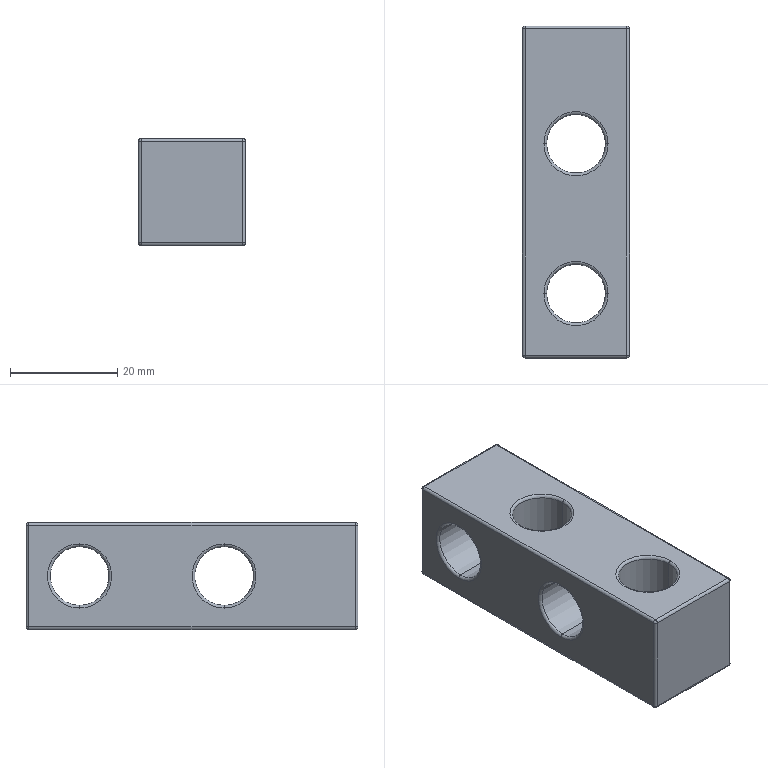Part | SolidWorks | features Extrusion 1, Fillet 1, ICE 1 | 1 solid | 50 faces | box 20 x 62 x 20 mm | volume 17160 mm3 | cylinder 20 | torus 16 | sphere 8 | plane 6 | commonest cylinder face diameters 1 x12 11 x8
STEP:
#1=CARTESIAN_POINT('',(-6.,-19.,10.));
#2=VERTEX_POINT('',#1);
#3=CARTESIAN_POINT('',(6.,-19.,10.));
#4=VERTEX_POINT('',#3);
#5=CARTESIAN_POINT('',(0.,-19.,10.));
#6=DIRECTION('',(0.,0.,-1.));
#7=DIRECTION('',(1.,0.,0.));
#8=AXIS2_PLACEMENT_3D('',#5,#6,#7);
#9=CIRCLE('',#8,6.);
#10=EDGE_CURVE('',#2,#4,#9,.T.);
#11=ORIENTED_EDGE('',*,*,#10,.F.);
#12=CARTESIAN_POINT('',(-5.5,-19.,9.5));
#13=VERTEX_POINT('',#12);
#14=CARTESIAN_POINT('',(-6.,-19.,9.5));
#15=DIRECTION('',(0.,1.,0.));
#16=DIRECTION('',(-1.,0.,0.));
#17=AXIS2_PLACEMENT_3D('',#14,#15,#16);
#18=CIRCLE('',#17,0.5);
#19=EDGE_CURVE('',#2,#13,#18,.T.);
#20=ORIENTED_EDGE('',*,*,#19,.T.);
#21=CARTESIAN_POINT('',(5.5,-19.,9.5));
#22=VERTEX_POINT('',#21);
#23=CARTESIAN_POINT('',(0.,-19.,9.5));
#24=DIRECTION('',(0.,0.,1.));
#25=DIRECTION('',(1.,0.,0.));
#26=AXIS2_PLACEMENT_3D('',#23,#24,#25);
#27=CIRCLE('',#26,5.5);
#28=EDGE_CURVE('',#22,#13,#27,.T.);
#29=ORIENTED_EDGE('',*,*,#28,.F.);
#30=CARTESIAN_POINT('',(6.,-19.,9.5));
#31=DIRECTION('',(0.,-1.,0.));
#32=DIRECTION('',(0.,0.,-1.));
#33=AXIS2_PLACEMENT_3D('',#30,#31,#32);
#34=CIRCLE('',#33,0.5);
#35=EDGE_CURVE('',#4,#22,#34,.T.);
#36=ORIENTED_EDGE('',*,*,#35,.F.);
#37=EDGE_LOOP('',(#11,#20,#29,#36));
#38=FACE_OUTER_BOUND('',#37,.T.);
#39=CARTESIAN_POINT('',(0.,-19.,9.5));
#40=DIRECTION('',(0.,0.,1.));
#41=DIRECTION('',(1.,0.,0.));
#42=AXIS2_PLACEMENT_3D('',#39,#40,#41);
#43=TOROIDAL_SURFACE('',#42,6.,0.5);
#44=ADVANCED_FACE('',(#38),#43,.T.);
#45=CARTESIAN_POINT('',(-6.,9.,10.));
#46=VERTEX_POINT('',#45);
#47=CARTESIAN_POINT('',(6.,9.,10.));
#48=VERTEX_POINT('',#47);
#49=CARTESIAN_POINT('',(0.,9.,10.));
#50=DIRECTION('',(0.,0.,-1.));
#51=DIRECTION('',(1.,0.,0.));
#52=AXIS2_PLACEMENT_3D('',#49,#50,#51);
#53=CIRCLE('',#52,6.);
#54=EDGE_CURVE('',#46,#48,#53,.T.);
#55=ORIENTED_EDGE('',*,*,#54,.F.);
#56=CARTESIAN_POINT('',(-5.5,9.,9.5));
#57=VERTEX_POINT('',#56);
#58=CARTESIAN_POINT('',(-6.,9.,9.5));
#59=DIRECTION('',(0.,1.,0.));
#60=DIRECTION('',(-1.,0.,0.));
#61=AXIS2_PLACEMENT_3D('',#58,#59,#60);
#62=CIRCLE('',#61,0.5);
#63=EDGE_CURVE('',#46,#57,#62,.T.);
#64=ORIENTED_EDGE('',*,*,#63,.T.);
#65=CARTESIAN_POINT('',(5.5,9.,9.5));
#66=VERTEX_POINT('',#65);
#67=CARTESIAN_POINT('',(0.,9.,9.5));
#68=DIRECTION('',(0.,0.,1.));
#69=DIRECTION('',(1.,0.,0.));
#70=AXIS2_PLACEMENT_3D('',#67,#68,#69);
#71=CIRCLE('',#70,5.5);
#72=EDGE_CURVE('',#66,#57,#71,.T.);
#73=ORIENTED_EDGE('',*,*,#72,.F.);
#74=CARTESIAN_POINT('',(6.,9.,9.5));
#75=DIRECTION('',(0.,-1.,0.));
#76=DIRECTION('',(0.,0.,-1.));
#77=AXIS2_PLACEMENT_3D('',#74,#75,#76);
#78=CIRCLE('',#77,0.5);
#79=EDGE_CURVE('',#48,#66,#78,.T.);
#80=ORIENTED_EDGE('',*,*,#79,.F.);
#81=EDGE_LOOP('',(#55,#64,#73,#80));
#82=FACE_OUTER_BOUND('',#81,.T.);
#83=CARTESIAN_POINT('',(0.,9.,9.5));
#84=DIRECTION('',(0.,0.,1.));
#85=DIRECTION('',(1.,0.,0.));
#86=AXIS2_PLACEMENT_3D('',#83,#84,#85);
#87=TOROIDAL_SURFACE('',#86,6.,0.5);
#88=ADVANCED_FACE('',(#82),#87,.T.);
#89=CARTESIAN_POINT('',(9.5,-6.,-5.5));
#90=VERTEX_POINT('',#89);
#91=CARTESIAN_POINT('',(9.5,-6.,5.5));
#92=VERTEX_POINT('',#91);
#93=CARTESIAN_POINT('',(9.5,-6.,0.));
#94=DIRECTION('',(1.,0.,0.));
#95=DIRECTION('',(0.,0.,1.));
#96=AXIS2_PLACEMENT_3D('',#93,#94,#95);
#97=CIRCLE('',#96,5.5);
#98=EDGE_CURVE('',#90,#92,#97,.T.);
#99=ORIENTED_EDGE('',*,*,#98,.F.);
#100=CARTESIAN_POINT('',(10.,-6.,-6.));
#101=VERTEX_POINT('',#100);
#102=CARTESIAN_POINT('',(9.5,-6.,-6.));
#103=DIRECTION('',(0.,1.,0.));
#104=DIRECTION('',(0.,0.,1.));
#105=AXIS2_PLACEMENT_3D('',#102,#103,#104);
#106=CIRCLE('',#105,0.5);
#107=EDGE_CURVE('',#90,#101,#106,.T.);
#108=ORIENTED_EDGE('',*,*,#107,.T.);
#109=CARTESIAN_POINT('',(10.,-6.,6.));
#110=VERTEX_POINT('',#109);
#111=CARTESIAN_POINT('',(10.,-6.,0.));
#112=DIRECTION('',(-1.,0.,0.));
#113=DIRECTION('',(0.,0.,1.));
#114=AXIS2_PLACEMENT_3D('',#111,#112,#113);
#115=CIRCLE('',#114,6.);
#116=EDGE_CURVE('',#110,#101,#115,.T.);
#117=ORIENTED_EDGE('',*,*,#116,.F.);
#118=CARTESIAN_POINT('',(9.5,-6.,6.));
#119=DIRECTION('',(0.,-1.,0.));
#120=DIRECTION('',(0.,0.,-1.));
#121=AXIS2_PLACEMENT_3D('',#118,#119,#120);
#122=CIRCLE('',#121,0.5);
#123=EDGE_CURVE('',#92,#110,#122,.T.);
#124=ORIENTED_EDGE('',*,*,#123,.F.);
#125=EDGE_LOOP('',(#99,#108,#117,#124));
#126=FACE_OUTER_BOUND('',#125,.T.);
#127=CARTESIAN_POINT('',(9.5,-6.,0.));
#128=DIRECTION('',(-1.,0.,0.));
#129=DIRECTION('',(0.,0.,1.));
#130=AXIS2_PLACEMENT_3D('',#127,#128,#129);
#131=TOROIDAL_SURFACE('',#130,6.,0.5);
#132=ADVANCED_FACE('',(#126),#131,.T.);
#133=CARTESIAN_POINT('',(9.5,21.,-5.5));
#134=VERTEX_POINT('',#133);
#135=CARTESIAN_POINT('',(9.5,21.,5.5));
#136=VERTEX_POINT('',#135);
#137=CARTESIAN_POINT('',(9.5,21.,0.));
#138=DIRECTION('',(1.,0.,0.));
#139=DIRECTION('',(0.,0.,1.));
#140=AXIS2_PLACEMENT_3D('',#137,#138,#139);
#141=CIRCLE('',#140,5.5);
#142=EDGE_CURVE('',#134,#136,#141,.T.);
#143=ORIENTED_EDGE('',*,*,#142,.F.);
#144=CARTESIAN_POINT('',(10.,21.,-6.));
#145=VERTEX_POINT('',#144);
#146=CARTESIAN_POINT('',(9.5,21.,-6.));
#147=DIRECTION('',(0.,1.,0.));
#148=DIRECTION('',(0.,0.,1.));
#149=AXIS2_PLACEMENT_3D('',#146,#147,#148);
#150=CIRCLE('',#149,0.5);
#151=EDGE_CURVE('',#134,#145,#150,.T.);
#152=ORIENTED_EDGE('',*,*,#151,.T.);
#153=CARTESIAN_POINT('',(10.,21.,6.));
#154=VERTEX_POINT('',#153);
#155=CARTESIAN_POINT('',(10.,21.,0.));
#156=DIRECTION('',(-1.,0.,0.));
#157=DIRECTION('',(0.,0.,1.));
#158=AXIS2_PLACEMENT_3D('',#155,#156,#157);
#159=CIRCLE('',#158,6.);
#160=EDGE_CURVE('',#154,#145,#159,.T.);
#161=ORIENTED_EDGE('',*,*,#160,.F.);
#162=CARTESIAN_POINT('',(9.5,21.,6.));
#163=DIRECTION('',(0.,-1.,0.));
#164=DIRECTION('',(0.,0.,-1.));
#165=AXIS2_PLACEMENT_3D('',#162,#163,#164);
#166=CIRCLE('',#165,0.5);
#167=EDGE_CURVE('',#136,#154,#166,.T.);
#168=ORIENTED_EDGE('',*,*,#167,.F.);
#169=EDGE_LOOP('',(#143,#152,#161,#168));
#170=FACE_OUTER_BOUND('',#169,.T.);
#171=CARTESIAN_POINT('',(9.5,21.,0.));
#172=DIRECTION('',(-1.,0.,0.));
#173=DIRECTION('',(0.,0.,1.));
#174=AXIS2_PLACEMENT_3D('',#171,#172,#173);
#175=TOROIDAL_SURFACE('',#174,6.,0.5);
#176=ADVANCED_FACE('',(#170),#175,.T.);
#177=CARTESIAN_POINT('',(-5.5,-19.,-9.5));
#178=VERTEX_POINT('',#177);
#179=CARTESIAN_POINT('',(5.5,-19.,-9.5));
#180=VERTEX_POINT('',#179);
#181=CARTESIAN_POINT('',(0.,-19.,-9.5));
#182=DIRECTION('',(0.,0.,-1.));
#183=DIRECTION('',(1.,0.,0.));
#184=AXIS2_PLACEMENT_3D('',#181,#182,#183);
#185=CIRCLE('',#184,5.5);
#186=EDGE_CURVE('',#178,#180,#185,.T.);
#187=ORIENTED_EDGE('',*,*,#186,.F.);
#188=CARTESIAN_POINT('',(-6.,-19.,-10.));
#189=VERTEX_POINT('',#188);
#190=CARTESIAN_POINT('',(-6.,-19.,-9.5));
#191=DIRECTION('',(0.,1.,0.));
#192=DIRECTION('',(-1.,0.,0.));
#193=AXIS2_PLACEMENT_3D('',#190,#191,#192);
#194=CIRCLE('',#193,0.5);
#195=EDGE_CURVE('',#178,#189,#194,.T.);
#196=ORIENTED_EDGE('',*,*,#195,.T.);
#197=CARTESIAN_POINT('',(6.,-19.,-10.));
#198=VERTEX_POINT('',#197);
#199=CARTESIAN_POINT('',(0.,-19.,-10.));
#200=DIRECTION('',(0.,0.,1.));
#201=DIRECTION('',(1.,0.,0.));
#202=AXIS2_PLACEMENT_3D('',#199,#200,#201);
#203=CIRCLE('',#202,6.);
#204=EDGE_CURVE('',#198,#189,#203,.T.);
#205=ORIENTED_EDGE('',*,*,#204,.F.);
#206=CARTESIAN_POINT('',(6.,-19.,-9.5));
#207=DIRECTION('',(0.,-1.,0.));
#208=DIRECTION('',(0.,0.,-1.));
#209=AXIS2_PLACEMENT_3D('',#206,#207,#208);
#210=CIRCLE('',#209,0.5);
#211=EDGE_CURVE('',#180,#198,#210,.T.);
#212=ORIENTED_EDGE('',*,*,#211,.F.);
#213=EDGE_LOOP('',(#187,#196,#205,#212));
#214=FACE_OUTER_BOUND('',#213,.T.);
#215=CARTESIAN_POINT('',(0.,-19.,-9.5));
#216=DIRECTION('',(0.,0.,1.));
#217=DIRECTION('',(1.,0.,0.));
#218=AXIS2_PLACEMENT_3D('',#215,#216,#217);
#219=TOROIDAL_SURFACE('',#218,6.,0.5);
#220=ADVANCED_FACE('',(#214),#219,.T.);
#221=CARTESIAN_POINT('',(-5.5,9.,-9.5));
#222=VERTEX_POINT('',#221);
#223=CARTESIAN_POINT('',(5.5,9.,-9.5));
#224=VERTEX_POINT('',#223);
#225=CARTESIAN_POINT('',(0.,9.,-9.5));
#226=DIRECTION('',(0.,0.,-1.));
#227=DIRECTION('',(1.,0.,0.));
#228=AXIS2_PLACEMENT_3D('',#225,#226,#227);
#229=CIRCLE('',#228,5.5);
#230=EDGE_CURVE('',#222,#224,#229,.T.);
#231=ORIENTED_EDGE('',*,*,#230,.F.);
#232=CARTESIAN_POINT('',(-6.,9.,-10.));
#233=VERTEX_POINT('',#232);
#234=CARTESIAN_POINT('',(-6.,9.,-9.5));
#235=DIRECTION('',(0.,1.,0.));
#236=DIRECTION('',(-1.,0.,0.));
#237=AXIS2_PLACEMENT_3D('',#234,#235,#236);
#238=CIRCLE('',#237,0.5);
#239=EDGE_CURVE('',#222,#233,#238,.T.);
#240=ORIENTED_EDGE('',*,*,#239,.T.);
#241=CARTESIAN_POINT('',(6.,9.,-10.));
#242=VERTEX_POINT('',#241);
#243=CARTESIAN_POINT('',(0.,9.,-10.));
#244=DIRECTION('',(0.,0.,1.));
#245=DIRECTION('',(1.,0.,0.));
#246=AXIS2_PLACEMENT_3D('',#243,#244,#245);
#247=CIRCLE('',#246,6.);
#248=EDGE_CURVE('',#242,#233,#247,.T.);
#249=ORIENTED_EDGE('',*,*,#248,.F.);
#250=CARTESIAN_POINT('',(6.,9.,-9.5));
#251=DIRECTION('',(0.,-1.,0.));
#252=DIRECTION('',(0.,0.,-1.));
#253=AXIS2_PLACEMENT_3D('',#250,#251,#252);
#254=CIRCLE('',#253,0.5);
#255=EDGE_CURVE('',#224,#242,#254,.T.);
#256=ORIENTED_EDGE('',*,*,#255,.F.);
#257=EDGE_LOOP('',(#231,#240,#249,#256));
#258=FACE_OUTER_BOUND('',#257,.T.);
#259=CARTESIAN_POINT('',(0.,9.,-9.5));
#260=DIRECTION('',(0.,0.,1.));
#261=DIRECTION('',(1.,0.,0.));
#262=AXIS2_PLACEMENT_3D('',#259,#260,#261);
#263=TOROIDAL_SURFACE('',#262,6.,0.5);
#264=ADVANCED_FACE('',(#258),#263,.T.);
#265=CARTESIAN_POINT('',(-9.5,-6.,5.5));
#266=VERTEX_POINT('',#265);
#267=CARTESIAN_POINT('',(-9.5,-6.,-5.5));
#268=VERTEX_POINT('',#267);
#269=CARTESIAN_POINT('',(-9.5,-6.,0.));
#270=DIRECTION('',(-1.,0.,0.));
#271=DIRECTION('',(0.,0.,-1.));
#272=AXIS2_PLACEMENT_3D('',#269,#270,#271);
#273=CIRCLE('',#272,5.5);
#274=EDGE_CURVE('',#266,#268,#273,.T.);
#275=ORIENTED_EDGE('',*,*,#274,.F.);
#276=CARTESIAN_POINT('',(-10.,-6.,6.));
#277=VERTEX_POINT('',#276);
#278=CARTESIAN_POINT('',(-9.5,-6.,6.));
#279=DIRECTION('',(0.,1.,0.));
#280=DIRECTION('',(0.,0.,1.));
#281=AXIS2_PLACEMENT_3D('',#278,#279,#280);
#282=CIRCLE('',#281,0.5);
#283=EDGE_CURVE('',#266,#277,#282,.T.);
#284=ORIENTED_EDGE('',*,*,#283,.T.);
#285=CARTESIAN_POINT('',(-10.,-6.,-6.));
#286=VERTEX_POINT('',#285);
#287=CARTESIAN_POINT('',(-10.,-6.,0.));
#288=DIRECTION('',(1.,0.,0.));
#289=DIRECTION('',(0.,0.,-1.));
#290=AXIS2_PLACEMENT_3D('',#287,#288,#289);
#291=CIRCLE('',#290,6.);
#292=EDGE_CURVE('',#286,#277,#291,.T.);
#293=ORIENTED_EDGE('',*,*,#292,.F.);
#294=CARTESIAN_POINT('',(-9.5,-6.,-6.));
#295=DIRECTION('',(0.,-1.,0.));
#296=DIRECTION('',(0.,0.,-1.));
#297=AXIS2_PLACEMENT_3D('',#294,#295,#296);
#298=CIRCLE('',#297,0.5);
#299=EDGE_CURVE('',#268,#286,#298,.T.);
#300=ORIENTED_EDGE('',*,*,#299,.F.);
#301=EDGE_LOOP('',(#275,#284,#293,#300));
#302=FACE_OUTER_BOUND('',#301,.T.);
#303=CARTESIAN_POINT('',(-9.5,-6.,0.));
#304=DIRECTION('',(1.,0.,0.));
#305=DIRECTION('',(0.,0.,-1.));
#306=AXIS2_PLACEMENT_3D('',#303,#304,#305);
#307=TOROIDAL_SURFACE('',#306,6.,0.5);
#308=ADVANCED_FACE('',(#302),#307,.T.);
#309=CARTESIAN_POINT('',(-9.5,21.,5.5));
#310=VERTEX_POINT('',#309);
#311=CARTESIAN_POINT('',(-9.5,21.,-5.5));
#312=VERTEX_POINT('',#311);
#313=CARTESIAN_POINT('',(-9.5,21.,0.));
#314=DIRECTION('',(-1.,0.,0.));
#315=DIRECTION('',(0.,0.,-1.));
#316=AXIS2_PLACEMENT_3D('',#313,#314,#315);
#317=CIRCLE('',#316,5.5);
#318=EDGE_CURVE('',#310,#312,#317,.T.);
#319=ORIENTED_EDGE('',*,*,#318,.F.);
#320=CARTESIAN_POINT('',(-10.,21.,6.));
#321=VERTEX_POINT('',#320);
#322=CARTESIAN_POINT('',(-9.5,21.,6.));
#323=DIRECTION('',(0.,1.,0.));
#324=DIRECTION('',(0.,0.,1.));
#325=AXIS2_PLACEMENT_3D('',#322,#323,#324);
#326=CIRCLE('',#325,0.5);
#327=EDGE_CURVE('',#310,#321,#326,.T.);
#328=ORIENTED_EDGE('',*,*,#327,.T.);
#329=CARTESIAN_POINT('',(-10.,21.,-6.));
#330=VERTEX_POINT('',#329);
#331=CARTESIAN_POINT('',(-10.,21.,0.));
#332=DIRECTION('',(1.,0.,0.));
#333=DIRECTION('',(0.,0.,-1.));
#334=AXIS2_PLACEMENT_3D('',#331,#332,#333);
#335=CIRCLE('',#334,6.);
#336=EDGE_CURVE('',#330,#321,#335,.T.);
#337=ORIENTED_EDGE('',*,*,#336,.F.);
#338=CARTESIAN_POINT('',(-9.5,21.,-6.));
#339=DIRECTION('',(0.,-1.,0.));
#340=DIRECTION('',(0.,0.,-1.));
#341=AXIS2_PLACEMENT_3D('',#338,#339,#340);
#342=CIRCLE('',#341,0.5);
#343=EDGE_CURVE('',#312,#330,#342,.T.);
#344=ORIENTED_EDGE('',*,*,#343,.F.);
#345=EDGE_LOOP('',(#319,#328,#337,#344));
#346=FACE_OUTER_BOUND('',#345,.T.);
#347=CARTESIAN_POINT('',(-9.5,21.,0.));
#348=DIRECTION('',(1.,0.,0.));
#349=DIRECTION('',(0.,0.,-1.));
#350=AXIS2_PLACEMENT_3D('',#347,#348,#349);
#351=TOROIDAL_SURFACE('',#350,6.,0.5);
#352=ADVANCED_FACE('',(#346),#351,.T.);
#353=CARTESIAN_POINT('',(-9.5,-6.,0.));
#354=DIRECTION('',(-1.,0.,0.));
#355=DIRECTION('',(0.,0.,-1.));
#356=AXIS2_PLACEMENT_3D('',#353,#354,#355);
#357=CIRCLE('',#356,5.5);
#358=EDGE_CURVE('',#268,#266,#357,.T.);
#359=ORIENTED_EDGE('',*,*,#358,.T.);
#360=CARTESIAN_POINT('',(-10.,-6.,5.5));
#361=DIRECTION('',(1.,0.,0.));
#362=VECTOR('',#361,1000.);
#363=LINE('',#360,#362);
#364=EDGE_CURVE('',#266,#92,#363,.T.);
#365=ORIENTED_EDGE('',*,*,#364,.T.);
#366=CARTESIAN_POINT('',(9.5,-6.,0.));
#367=DIRECTION('',(1.,0.,0.));
#368=DIRECTION('',(0.,0.,1.));
#369=AXIS2_PLACEMENT_3D('',#366,#367,#368);
#370=CIRCLE('',#369,5.5);
#371=EDGE_CURVE('',#92,#90,#370,.T.);
#372=ORIENTED_EDGE('',*,*,#371,.T.);
#373=CARTESIAN_POINT('',(-10.,-6.,-5.5));
#374=DIRECTION('',(1.,0.,0.));
#375=VECTOR('',#374,1000.);
#376=LINE('',#373,#375);
#377=EDGE_CURVE('',#268,#90,#376,.T.);
#378=ORIENTED_EDGE('',*,*,#377,.F.);
#379=EDGE_LOOP('',(#359,#365,#372,#378));
#380=FACE_OUTER_BOUND('',#379,.T.);
#381=CARTESIAN_POINT('',(-10.,-6.,0.));
#382=DIRECTION('',(1.,0.,0.));
#383=DIRECTION('',(0.,0.,-1.));
#384=AXIS2_PLACEMENT_3D('',#381,#382,#383);
#385=CYLINDRICAL_SURFACE('',#384,5.5);
#386=ADVANCED_FACE('',(#380),#385,.F.);
#387=CARTESIAN_POINT('',(-9.5,21.,0.));
#388=DIRECTION('',(-1.,0.,0.));
#389=DIRECTION('',(0.,0.,-1.));
#390=AXIS2_PLACEMENT_3D('',#387,#388,#389);
#391=CIRCLE('',#390,5.5);
#392=EDGE_CURVE('',#312,#310,#391,.T.);
#393=ORIENTED_EDGE('',*,*,#392,.T.);
#394=CARTESIAN_POINT('',(-10.,21.,5.5));
#395=DIRECTION('',(1.,0.,0.));
#396=VECTOR('',#395,1000.);
#397=LINE('',#394,#396);
#398=EDGE_CURVE('',#310,#136,#397,.T.);
#399=ORIENTED_EDGE('',*,*,#398,.T.);
#400=CARTESIAN_POINT('',(9.5,21.,0.));
#401=DIRECTION('',(1.,0.,0.));
#402=DIRECTION('',(0.,0.,1.));
#403=AXIS2_PLACEMENT_3D('',#400,#401,#402);
#404=CIRCLE('',#403,5.5);
#405=EDGE_CURVE('',#136,#134,#404,.T.);
#406=ORIENTED_EDGE('',*,*,#405,.T.);
#407=CARTESIAN_POINT('',(-10.,21.,-5.5));
#408=DIRECTION('',(1.,0.,0.));
#409=VECTOR('',#408,1000.);
#410=LINE('',#407,#409);
#411=EDGE_CURVE('',#312,#134,#410,.T.);
#412=ORIENTED_EDGE('',*,*,#411,.F.);
#413=EDGE_LOOP('',(#393,#399,#406,#412));
#414=FACE_OUTER_BOUND('',#413,.T.);
#415=CARTESIAN_POINT('',(-10.,21.,0.));
#416=DIRECTION('',(1.,0.,0.));
#417=DIRECTION('',(0.,0.,-1.));
#418=AXIS2_PLACEMENT_3D('',#415,#416,#417);
#419=CYLINDRICAL_SURFACE('',#418,5.5);
#420=ADVANCED_FACE('',(#414),#419,.F.);
#421=CARTESIAN_POINT('',(0.,9.,9.5));
#422=DIRECTION('',(0.,0.,1.));
#423=DIRECTION('',(1.,0.,0.));
#424=AXIS2_PLACEMENT_3D('',#421,#422,#423);
#425=CIRCLE('',#424,5.5);
#426=EDGE_CURVE('',#57,#66,#425,.T.);
#427=ORIENTED_EDGE('',*,*,#426,.T.);
#428=CARTESIAN_POINT('',(5.5,9.,10.));
#429=DIRECTION('',(0.,0.,-1.));
#430=VECTOR('',#429,1000.);
#431=LINE('',#428,#430);
#432=EDGE_CURVE('',#66,#224,#431,.T.);
#433=ORIENTED_EDGE('',*,*,#432,.T.);
#434=CARTESIAN_POINT('',(0.,9.,-9.5));
#435=DIRECTION('',(0.,0.,-1.));
#436=DIRECTION('',(1.,0.,0.));
#437=AXIS2_PLACEMENT_3D('',#434,#435,#436);
#438=CIRCLE('',#437,5.5);
#439=EDGE_CURVE('',#224,#222,#438,.T.);
#440=ORIENTED_EDGE('',*,*,#439,.T.);
#441=CARTESIAN_POINT('',(-5.5,9.,10.));
#442=DIRECTION('',(0.,0.,-1.));
#443=VECTOR('',#442,1000.);
#444=LINE('',#441,#443);
#445=EDGE_CURVE('',#57,#222,#444,.T.);
#446=ORIENTED_EDGE('',*,*,#445,.F.);
#447=EDGE_LOOP('',(#427,#433,#440,#446));
#448=FACE_OUTER_BOUND('',#447,.T.);
#449=CARTESIAN_POINT('',(0.,9.,10.));
#450=DIRECTION('',(0.,0.,-1.));
#451=DIRECTION('',(-1.,0.,0.));
#452=AXIS2_PLACEMENT_3D('',#449,#450,#451);
#453=CYLINDRICAL_SURFACE('',#452,5.5);
#454=ADVANCED_FACE('',(#448),#453,.F.);
#455=CARTESIAN_POINT('',(0.,-19.,9.5));
#456=DIRECTION('',(0.,0.,1.));
#457=DIRECTION('',(1.,0.,0.));
#458=AXIS2_PLACEMENT_3D('',#455,#456,#457);
#459=CIRCLE('',#458,5.5);
#460=EDGE_CURVE('',#13,#22,#459,.T.);
#461=ORIENTED_EDGE('',*,*,#460,.T.);
#462=CARTESIAN_POINT('',(5.5,-19.,10.));
#463=DIRECTION('',(0.,0.,-1.));
#464=VECTOR('',#463,1000.);
#465=LINE('',#462,#464);
#466=EDGE_CURVE('',#22,#180,#465,.T.);
#467=ORIENTED_EDGE('',*,*,#466,.T.);
#468=CARTESIAN_POINT('',(0.,-19.,-9.5));
#469=DIRECTION('',(0.,0.,-1.));
#470=DIRECTION('',(1.,0.,0.));
#471=AXIS2_PLACEMENT_3D('',#468,#469,#470);
#472=CIRCLE('',#471,5.5);
#473=EDGE_CURVE('',#180,#178,#472,.T.);
#474=ORIENTED_EDGE('',*,*,#473,.T.);
#475=CARTESIAN_POINT('',(-5.5,-19.,10.));
#476=DIRECTION('',(0.,0.,-1.));
#477=VECTOR('',#476,1000.);
#478=LINE('',#475,#477);
#479=EDGE_CURVE('',#13,#178,#478,.T.);
#480=ORIENTED_EDGE('',*,*,#479,.F.);
#481=EDGE_LOOP('',(#461,#467,#474,#480));
#482=FACE_OUTER_BOUND('',#481,.T.);
#483=CARTESIAN_POINT('',(0.,-19.,10.));
#484=DIRECTION('',(0.,0.,-1.));
#485=DIRECTION('',(-1.,0.,0.));
#486=AXIS2_PLACEMENT_3D('',#483,#484,#485);
#487=CYLINDRICAL_SURFACE('',#486,5.5);
#488=ADVANCED_FACE('',(#482),#487,.F.);
#489=CARTESIAN_POINT('',(0.,9.,10.));
#490=DIRECTION('',(0.,0.,-1.));
#491=DIRECTION('',(1.,0.,0.));
#492=AXIS2_PLACEMENT_3D('',#489,#490,#491);
#493=CIRCLE('',#492,6.);
#494=EDGE_CURVE('',#48,#46,#493,.T.);
#495=ORIENTED_EDGE('',*,*,#494,.T.);
#496=ORIENTED_EDGE('',*,*,#54,.T.);
#497=EDGE_LOOP('',(#495,#496));
#498=FACE_BOUND('',#497,.T.);
#499=CARTESIAN_POINT('',(0.,-19.,10.));
#500=DIRECTION('',(0.,0.,-1.));
#501=DIRECTION('',(1.,0.,0.));
#502=AXIS2_PLACEMENT_3D('',#499,#500,#501);
#503=CIRCLE('',#502,6.);
#504=EDGE_CURVE('',#4,#2,#503,.T.);
#505=ORIENTED_EDGE('',*,*,#504,.T.);
#506=ORIENTED_EDGE('',*,*,#10,.T.);
#507=EDGE_LOOP('',(#505,#506));
#508=FACE_BOUND('',#507,.T.);
#509=CARTESIAN_POINT('',(-9.5,-30.5,10.));
#510=VERTEX_POINT('',#509);
#511=CARTESIAN_POINT('',(9.5,-30.5,10.));
#512=VERTEX_POINT('',#511);
#513=CARTESIAN_POINT('',(10.,-30.5,10.));
#514=DIRECTION('',(1.,0.,0.));
#515=VECTOR('',#514,1000.);
#516=LINE('',#513,#515);
#517=EDGE_CURVE('',#510,#512,#516,.T.);
#518=ORIENTED_EDGE('',*,*,#517,.T.);
#519=CARTESIAN_POINT('',(9.5,30.5,10.));
#520=VERTEX_POINT('',#519);
#521=CARTESIAN_POINT('',(9.5,31.,10.));
#522=DIRECTION('',(0.,1.,0.));
#523=VECTOR('',#522,1000.);
#524=LINE('',#521,#523);
#525=EDGE_CURVE('',#512,#520,#524,.T.);
#526=ORIENTED_EDGE('',*,*,#525,.T.);
#527=CARTESIAN_POINT('',(-9.5,30.5,10.));
#528=VERTEX_POINT('',#527);
#529=CARTESIAN_POINT('',(-10.,30.5,10.));
#530=DIRECTION('',(-1.,0.,0.));
#531=VECTOR('',#530,1000.);
#532=LINE('',#529,#531);
#533=EDGE_CURVE('',#520,#528,#532,.T.);
#534=ORIENTED_EDGE('',*,*,#533,.T.);
#535=CARTESIAN_POINT('',(-9.5,-31.,10.));
#536=DIRECTION('',(0.,-1.,0.));
#537=VECTOR('',#536,1000.);
#538=LINE('',#535,#537);
#539=EDGE_CURVE('',#528,#510,#538,.T.);
#540=ORIENTED_EDGE('',*,*,#539,.T.);
#541=EDGE_LOOP('',(#518,#526,#534,#540));
#542=FACE_OUTER_BOUND('',#541,.T.);
#543=CARTESIAN_POINT('',(0.,0.,10.));
#544=DIRECTION('',(0.,0.,1.));
#545=DIRECTION('',(1.,0.,0.));
#546=AXIS2_PLACEMENT_3D('',#543,#544,#545);
#547=PLANE('',#546);
#548=ADVANCED_FACE('',(#498,#508,#542),#547,.T.);
#549=ORIENTED_EDGE('',*,*,#248,.T.);
#550=CARTESIAN_POINT('',(0.,9.,-10.));
#551=DIRECTION('',(0.,0.,1.));
#552=DIRECTION('',(1.,0.,0.));
#553=AXIS2_PLACEMENT_3D('',#550,#551,#552);
#554=CIRCLE('',#553,6.);
#555=EDGE_CURVE('',#233,#242,#554,.T.);
#556=ORIENTED_EDGE('',*,*,#555,.T.);
#557=EDGE_LOOP('',(#549,#556));
#558=FACE_BOUND('',#557,.T.);
#559=ORIENTED_EDGE('',*,*,#204,.T.);
#560=CARTESIAN_POINT('',(0.,-19.,-10.));
#561=DIRECTION('',(0.,0.,1.));
#562=DIRECTION('',(1.,0.,0.));
#563=AXIS2_PLACEMENT_3D('',#560,#561,#562);
#564=CIRCLE('',#563,6.);
#565=EDGE_CURVE('',#189,#198,#564,.T.);
#566=ORIENTED_EDGE('',*,*,#565,.T.);
#567=EDGE_LOOP('',(#559,#566));
#568=FACE_BOUND('',#567,.T.);
#569=CARTESIAN_POINT('',(9.5,30.5,-10.));
#570=VERTEX_POINT('',#569);
#571=CARTESIAN_POINT('',(9.5,-30.5,-10.));
#572=VERTEX_POINT('',#571);
#573=CARTESIAN_POINT('',(9.5,0.,-10.));
#574=DIRECTION('',(0.,-1.,0.));
#575=VECTOR('',#574,1000.);
#576=LINE('',#573,#575);
#577=EDGE_CURVE('',#570,#572,#576,.T.);
#578=ORIENTED_EDGE('',*,*,#577,.T.);
#579=CARTESIAN_POINT('',(-9.5,-30.5,-10.));
#580=VERTEX_POINT('',#579);
#581=CARTESIAN_POINT('',(0.,-30.5,-10.));
#582=DIRECTION('',(-1.,0.,0.));
#583=VECTOR('',#582,1000.);
#584=LINE('',#581,#583);
#585=EDGE_CURVE('',#572,#580,#584,.T.);
#586=ORIENTED_EDGE('',*,*,#585,.T.);
#587=CARTESIAN_POINT('',(-9.5,30.5,-10.));
#588=VERTEX_POINT('',#587);
#589=CARTESIAN_POINT('',(-9.5,0.,-10.));
#590=DIRECTION('',(0.,1.,0.));
#591=VECTOR('',#590,1000.);
#592=LINE('',#589,#591);
#593=EDGE_CURVE('',#580,#588,#592,.T.);
#594=ORIENTED_EDGE('',*,*,#593,.T.);
#595=CARTESIAN_POINT('',(0.,30.5,-10.));
#596=DIRECTION('',(1.,0.,0.));
#597=VECTOR('',#596,1000.);
#598=LINE('',#595,#597);
#599=EDGE_CURVE('',#588,#570,#598,.T.);
#600=ORIENTED_EDGE('',*,*,#599,.T.);
#601=EDGE_LOOP('',(#578,#586,#594,#600));
#602=FACE_OUTER_BOUND('',#601,.T.);
#603=CARTESIAN_POINT('',(0.,0.,-10.));
#604=DIRECTION('',(0.,0.,1.));
#605=DIRECTION('',(1.,0.,0.));
#606=AXIS2_PLACEMENT_3D('',#603,#604,#605);
#607=PLANE('',#606);
#608=ADVANCED_FACE('',(#558,#568,#602),#607,.F.);
#609=ORIENTED_EDGE('',*,*,#336,.T.);
#610=CARTESIAN_POINT('',(-10.,21.,0.));
#611=DIRECTION('',(1.,0.,0.));
#612=DIRECTION('',(0.,0.,-1.));
#613=AXIS2_PLACEMENT_3D('',#610,#611,#612);
#614=CIRCLE('',#613,6.);
#615=EDGE_CURVE('',#321,#330,#614,.T.);
#616=ORIENTED_EDGE('',*,*,#615,.T.);
#617=EDGE_LOOP('',(#609,#616));
#618=FACE_BOUND('',#617,.T.);
#619=ORIENTED_EDGE('',*,*,#292,.T.);
#620=CARTESIAN_POINT('',(-10.,-6.,0.));
#621=DIRECTION('',(1.,0.,0.));
#622=DIRECTION('',(0.,0.,-1.));
#623=AXIS2_PLACEMENT_3D('',#620,#621,#622);
#624=CIRCLE('',#623,6.);
#625=EDGE_CURVE('',#277,#286,#624,.T.);
#626=ORIENTED_EDGE('',*,*,#625,.T.);
#627=EDGE_LOOP('',(#619,#626));
#628=FACE_BOUND('',#627,.T.);
#629=CARTESIAN_POINT('',(-10.,30.5,-9.5));
#630=VERTEX_POINT('',#629);
#631=CARTESIAN_POINT('',(-10.,-30.5,-9.5));
#632=VERTEX_POINT('',#631);
#633=CARTESIAN_POINT('',(-10.,-31.,-9.5));
#634=DIRECTION('',(0.,-1.,0.));
#635=VECTOR('',#634,1000.);
#636=LINE('',#633,#635);
#637=EDGE_CURVE('',#630,#632,#636,.T.);
#638=ORIENTED_EDGE('',*,*,#637,.T.);
#639=CARTESIAN_POINT('',(-10.,-30.5,9.5));
#640=VERTEX_POINT('',#639);
#641=CARTESIAN_POINT('',(-10.,-30.5,10.));
#642=DIRECTION('',(0.,0.,1.));
#643=VECTOR('',#642,1000.);
#644=LINE('',#641,#643);
#645=EDGE_CURVE('',#632,#640,#644,.T.);
#646=ORIENTED_EDGE('',*,*,#645,.T.);
#647=CARTESIAN_POINT('',(-10.,30.5,9.5));
#648=VERTEX_POINT('',#647);
#649=CARTESIAN_POINT('',(-10.,31.,9.5));
#650=DIRECTION('',(0.,1.,0.));
#651=VECTOR('',#650,1000.);
#652=LINE('',#649,#651);
#653=EDGE_CURVE('',#640,#648,#652,.T.);
#654=ORIENTED_EDGE('',*,*,#653,.T.);
#655=CARTESIAN_POINT('',(-10.,30.5,10.));
#656=DIRECTION('',(0.,0.,-1.));
#657=VECTOR('',#656,1000.);
#658=LINE('',#655,#657);
#659=EDGE_CURVE('',#648,#630,#658,.T.);
#660=ORIENTED_EDGE('',*,*,#659,.T.);
#661=EDGE_LOOP('',(#638,#646,#654,#660));
#662=FACE_OUTER_BOUND('',#661,.T.);
#663=CARTESIAN_POINT('',(-10.,-31.,10.));
#664=DIRECTION('',(1.,0.,0.));
#665=DIRECTION('',(0.,0.,-1.));
#666=AXIS2_PLACEMENT_3D('',#663,#664,#665);
#667=PLANE('',#666);
#668=ADVANCED_FACE('',(#618,#628,#662),#667,.F.);
#669=CARTESIAN_POINT('',(9.5,-31.,9.5));
#670=VERTEX_POINT('',#669);
#671=CARTESIAN_POINT('',(-9.5,-31.,9.5));
#672=VERTEX_POINT('',#671);
#673=CARTESIAN_POINT('',(-10.,-31.,9.5));
#674=DIRECTION('',(-1.,0.,0.));
#675=VECTOR('',#674,1000.);
#676=LINE('',#673,#675);
#677=EDGE_CURVE('',#670,#672,#676,.T.);
#678=ORIENTED_EDGE('',*,*,#677,.T.);
#679=CARTESIAN_POINT('',(-9.5,-31.,-9.5));
#680=VERTEX_POINT('',#679);
#681=CARTESIAN_POINT('',(-9.5,-31.,10.));
#682=DIRECTION('',(0.,0.,-1.));
#683=VECTOR('',#682,1000.);
#684=LINE('',#681,#683);
#685=EDGE_CURVE('',#672,#680,#684,.T.);
#686=ORIENTED_EDGE('',*,*,#685,.T.);
#687=CARTESIAN_POINT('',(9.5,-31.,-9.5));
#688=VERTEX_POINT('',#687);
#689=CARTESIAN_POINT('',(10.,-31.,-9.5));
#690=DIRECTION('',(1.,0.,0.));
#691=VECTOR('',#690,1000.);
#692=LINE('',#689,#691);
#693=EDGE_CURVE('',#680,#688,#692,.T.);
#694=ORIENTED_EDGE('',*,*,#693,.T.);
#695=CARTESIAN_POINT('',(9.5,-31.,10.));
#696=DIRECTION('',(0.,0.,1.));
#697=VECTOR('',#696,1000.);
#698=LINE('',#695,#697);
#699=EDGE_CURVE('',#688,#670,#698,.T.);
#700=ORIENTED_EDGE('',*,*,#699,.T.);
#701=EDGE_LOOP('',(#678,#686,#694,#700));
#702=FACE_OUTER_BOUND('',#701,.T.);
#703=CARTESIAN_POINT('',(10.,-31.,10.));
#704=DIRECTION('',(0.,1.,0.));
#705=DIRECTION('',(0.,0.,1.));
#706=AXIS2_PLACEMENT_3D('',#703,#704,#705);
#707=PLANE('',#706);
#708=ADVANCED_FACE('',(#702),#707,.F.);
#709=ORIENTED_EDGE('',*,*,#160,.T.);
#710=CARTESIAN_POINT('',(10.,21.,0.));
#711=DIRECTION('',(-1.,0.,0.));
#712=DIRECTION('',(0.,0.,1.));
#713=AXIS2_PLACEMENT_3D('',#710,#711,#712);
#714=CIRCLE('',#713,6.);
#715=EDGE_CURVE('',#145,#154,#714,.T.);
#716=ORIENTED_EDGE('',*,*,#715,.T.);
#717=EDGE_LOOP('',(#709,#716));
#718=FACE_BOUND('',#717,.T.);
#719=ORIENTED_EDGE('',*,*,#116,.T.);
#720=CARTESIAN_POINT('',(10.,-6.,0.));
#721=DIRECTION('',(-1.,0.,0.));
#722=DIRECTION('',(0.,0.,1.));
#723=AXIS2_PLACEMENT_3D('',#720,#721,#722);
#724=CIRCLE('',#723,6.);
#725=EDGE_CURVE('',#101,#110,#724,.T.);
#726=ORIENTED_EDGE('',*,*,#725,.T.);
#727=EDGE_LOOP('',(#719,#726));
#728=FACE_BOUND('',#727,.T.);
#729=CARTESIAN_POINT('',(10.,30.5,9.5));
#730=VERTEX_POINT('',#729);
#731=CARTESIAN_POINT('',(10.,-30.5,9.5));
#732=VERTEX_POINT('',#731);
#733=CARTESIAN_POINT('',(10.,-31.,9.5));
#734=DIRECTION('',(0.,-1.,0.));
#735=VECTOR('',#734,1000.);
#736=LINE('',#733,#735);
#737=EDGE_CURVE('',#730,#732,#736,.T.);
#738=ORIENTED_EDGE('',*,*,#737,.T.);
#739=CARTESIAN_POINT('',(10.,-30.5,-9.5));
#740=VERTEX_POINT('',#739);
#741=CARTESIAN_POINT('',(10.,-30.5,10.));
#742=DIRECTION('',(0.,0.,-1.));
#743=VECTOR('',#742,1000.);
#744=LINE('',#741,#743);
#745=EDGE_CURVE('',#732,#740,#744,.T.);
#746=ORIENTED_EDGE('',*,*,#745,.T.);
#747=CARTESIAN_POINT('',(10.,30.5,-9.5));
#748=VERTEX_POINT('',#747);
#749=CARTESIAN_POINT('',(10.,-31.,-9.5));
#750=DIRECTION('',(0.,1.,0.));
#751=VECTOR('',#750,1000.);
#752=LINE('',#749,#751);
#753=EDGE_CURVE('',#740,#748,#752,.T.);
#754=ORIENTED_EDGE('',*,*,#753,.T.);
#755=CARTESIAN_POINT('',(10.,30.5,10.));
#756=DIRECTION('',(0.,0.,1.));
#757=VECTOR('',#756,1000.);
#758=LINE('',#755,#757);
#759=EDGE_CURVE('',#748,#730,#758,.T.);
#760=ORIENTED_EDGE('',*,*,#759,.T.);
#761=EDGE_LOOP('',(#738,#746,#754,#760));
#762=FACE_OUTER_BOUND('',#761,.T.);
#763=CARTESIAN_POINT('',(10.,-31.,10.));
#764=DIRECTION('',(-1.,0.,0.));
#765=DIRECTION('',(0.,0.,1.));
#766=AXIS2_PLACEMENT_3D('',#763,#764,#765);
#767=PLANE('',#766);
#768=ADVANCED_FACE('',(#718,#728,#762),#767,.F.);
#769=CARTESIAN_POINT('',(-9.5,31.,9.5));
#770=VERTEX_POINT('',#769);
#771=CARTESIAN_POINT('',(9.5,31.,9.5));
#772=VERTEX_POINT('',#771);
#773=CARTESIAN_POINT('',(10.,31.,9.5));
#774=DIRECTION('',(1.,0.,0.));
#775=VECTOR('',#774,1000.);
#776=LINE('',#773,#775);
#777=EDGE_CURVE('',#770,#772,#776,.T.);
#778=ORIENTED_EDGE('',*,*,#777,.T.);
#779=CARTESIAN_POINT('',(9.5,31.,-9.5));
#780=VERTEX_POINT('',#779);
#781=CARTESIAN_POINT('',(9.5,31.,10.));
#782=DIRECTION('',(0.,0.,-1.));
#783=VECTOR('',#782,1000.);
#784=LINE('',#781,#783);
#785=EDGE_CURVE('',#772,#780,#784,.T.);
#786=ORIENTED_EDGE('',*,*,#785,.T.);
#787=CARTESIAN_POINT('',(-9.5,31.,-9.5));
#788=VERTEX_POINT('',#787);
#789=CARTESIAN_POINT('',(10.,31.,-9.5));
#790=DIRECTION('',(-1.,0.,0.));
#791=VECTOR('',#790,1000.);
#792=LINE('',#789,#791);
#793=EDGE_CURVE('',#780,#788,#792,.T.);
#794=ORIENTED_EDGE('',*,*,#793,.T.);
#795=CARTESIAN_POINT('',(-9.5,31.,10.));
#796=DIRECTION('',(0.,0.,1.));
#797=VECTOR('',#796,1000.);
#798=LINE('',#795,#797);
#799=EDGE_CURVE('',#788,#770,#798,.T.);
#800=ORIENTED_EDGE('',*,*,#799,.T.);
#801=EDGE_LOOP('',(#778,#786,#794,#800));
#802=FACE_OUTER_BOUND('',#801,.T.);
#803=CARTESIAN_POINT('',(10.,31.,10.));
#804=DIRECTION('',(0.,-1.,0.));
#805=DIRECTION('',(0.,0.,-1.));
#806=AXIS2_PLACEMENT_3D('',#803,#804,#805);
#807=PLANE('',#806);
#808=ADVANCED_FACE('',(#802),#807,.F.);
#809=ORIENTED_EDGE('',*,*,#466,.F.);
#810=ORIENTED_EDGE('',*,*,#28,.T.);
#811=ORIENTED_EDGE('',*,*,#479,.T.);
#812=ORIENTED_EDGE('',*,*,#186,.T.);
#813=EDGE_LOOP('',(#809,#810,#811,#812));
#814=FACE_OUTER_BOUND('',#813,.T.);
#815=CARTESIAN_POINT('',(0.,-19.,10.));
#816=DIRECTION('',(0.,0.,-1.));
#817=DIRECTION('',(-1.,0.,0.));
#818=AXIS2_PLACEMENT_3D('',#815,#816,#817);
#819=CYLINDRICAL_SURFACE('',#818,5.5);
#820=ADVANCED_FACE('',(#814),#819,.F.);
#821=ORIENTED_EDGE('',*,*,#432,.F.);
#822=ORIENTED_EDGE('',*,*,#72,.T.);
#823=ORIENTED_EDGE('',*,*,#445,.T.);
#824=ORIENTED_EDGE('',*,*,#230,.T.);
#825=EDGE_LOOP('',(#821,#822,#823,#824));
#826=FACE_OUTER_BOUND('',#825,.T.);
#827=CARTESIAN_POINT('',(0.,9.,10.));
#828=DIRECTION('',(0.,0.,-1.));
#829=DIRECTION('',(-1.,0.,0.));
#830=AXIS2_PLACEMENT_3D('',#827,#828,#829);
#831=CYLINDRICAL_SURFACE('',#830,5.5);
#832=ADVANCED_FACE('',(#826),#831,.F.);
#833=ORIENTED_EDGE('',*,*,#398,.F.);
#834=ORIENTED_EDGE('',*,*,#318,.T.);
#835=ORIENTED_EDGE('',*,*,#411,.T.);
#836=ORIENTED_EDGE('',*,*,#142,.T.);
#837=EDGE_LOOP('',(#833,#834,#835,#836));
#838=FACE_OUTER_BOUND('',#837,.T.);
#839=CARTESIAN_POINT('',(-10.,21.,0.));
#840=DIRECTION('',(1.,0.,0.));
#841=DIRECTION('',(0.,0.,-1.));
#842=AXIS2_PLACEMENT_3D('',#839,#840,#841);
#843=CYLINDRICAL_SURFACE('',#842,5.5);
#844=ADVANCED_FACE('',(#838),#843,.F.);
#845=ORIENTED_EDGE('',*,*,#364,.F.);
#846=ORIENTED_EDGE('',*,*,#274,.T.);
#847=ORIENTED_EDGE('',*,*,#377,.T.);
#848=ORIENTED_EDGE('',*,*,#98,.T.);
#849=EDGE_LOOP('',(#845,#846,#847,#848));
#850=FACE_OUTER_BOUND('',#849,.T.);
#851=CARTESIAN_POINT('',(-10.,-6.,0.));
#852=DIRECTION('',(1.,0.,0.));
#853=DIRECTION('',(0.,0.,-1.));
#854=AXIS2_PLACEMENT_3D('',#851,#852,#853);
#855=CYLINDRICAL_SURFACE('',#854,5.5);
#856=ADVANCED_FACE('',(#850),#855,.F.);
#857=CARTESIAN_POINT('',(9.5,30.5,9.5));
#858=DIRECTION('',(0.,0.,1.));
#859=DIRECTION('',(1.,0.,0.));
#860=AXIS2_PLACEMENT_3D('',#857,#858,#859);
#861=CIRCLE('',#860,0.5);
#862=EDGE_CURVE('',#730,#772,#861,.T.);
#863=ORIENTED_EDGE('',*,*,#862,.F.);
#864=ORIENTED_EDGE('',*,*,#759,.F.);
#865=CARTESIAN_POINT('',(9.5,30.5,-9.5));
#866=DIRECTION('',(0.,0.,-1.));
#867=DIRECTION('',(-1.,0.,0.));
#868=AXIS2_PLACEMENT_3D('',#865,#866,#867);
#869=CIRCLE('',#868,0.5);
#870=EDGE_CURVE('',#780,#748,#869,.T.);
#871=ORIENTED_EDGE('',*,*,#870,.F.);
#872=ORIENTED_EDGE('',*,*,#785,.F.);
#873=EDGE_LOOP('',(#863,#864,#871,#872));
#874=FACE_OUTER_BOUND('',#873,.T.);
#875=CARTESIAN_POINT('',(9.5,30.5,10.));
#876=DIRECTION('',(0.,0.,-1.));
#877=DIRECTION('',(-1.,0.,0.));
#878=AXIS2_PLACEMENT_3D('',#875,#876,#877);
#879=CYLINDRICAL_SURFACE('',#878,0.5);
#880=ADVANCED_FACE('',(#874),#879,.T.);
#881=CARTESIAN_POINT('',(9.5,30.5,9.5));
#882=DIRECTION('',(0.,-1.,0.));
#883=DIRECTION('',(0.,0.,1.));
#884=AXIS2_PLACEMENT_3D('',#881,#882,#883);
#885=CIRCLE('',#884,0.5);
#886=EDGE_CURVE('',#730,#520,#885,.T.);
#887=ORIENTED_EDGE('',*,*,#886,.F.);
#888=ORIENTED_EDGE('',*,*,#862,.T.);
#889=CARTESIAN_POINT('',(9.5,30.5,9.5));
#890=DIRECTION('',(-1.,0.,0.));
#891=DIRECTION('',(0.,0.,-1.));
#892=AXIS2_PLACEMENT_3D('',#889,#890,#891);
#893=CIRCLE('',#892,0.5);
#894=EDGE_CURVE('',#520,#772,#893,.T.);
#895=ORIENTED_EDGE('',*,*,#894,.F.);
#896=EDGE_LOOP('',(#887,#888,#895));
#897=FACE_OUTER_BOUND('',#896,.T.);
#898=CARTESIAN_POINT('',(9.5,30.5,9.5));
#899=DIRECTION('',(0.,1.,0.));
#900=DIRECTION('',(1.,0.,0.));
#901=AXIS2_PLACEMENT_3D('',#898,#899,#900);
#902=SPHERICAL_SURFACE('',#901,0.5);
#903=ADVANCED_FACE('',(#897),#902,.T.);
#904=CARTESIAN_POINT('',(9.5,30.5,-9.5));
#905=DIRECTION('',(-1.,0.,0.));
#906=DIRECTION('',(0.,0.,-1.));
#907=AXIS2_PLACEMENT_3D('',#904,#905,#906);
#908=CIRCLE('',#907,0.5);
#909=EDGE_CURVE('',#780,#570,#908,.T.);
#910=ORIENTED_EDGE('',*,*,#909,.F.);
#911=ORIENTED_EDGE('',*,*,#870,.T.);
#912=CARTESIAN_POINT('',(9.5,30.5,-9.5));
#913=DIRECTION('',(0.,-1.,0.));
#914=DIRECTION('',(0.,0.,1.));
#915=AXIS2_PLACEMENT_3D('',#912,#913,#914);
#916=CIRCLE('',#915,0.5);
#917=EDGE_CURVE('',#570,#748,#916,.T.);
#918=ORIENTED_EDGE('',*,*,#917,.F.);
#919=EDGE_LOOP('',(#910,#911,#918));
#920=FACE_OUTER_BOUND('',#919,.T.);
#921=CARTESIAN_POINT('',(9.5,30.5,-9.5));
#922=DIRECTION('',(0.,1.,0.));
#923=DIRECTION('',(1.,0.,0.));
#924=AXIS2_PLACEMENT_3D('',#921,#922,#923);
#925=SPHERICAL_SURFACE('',#924,0.5);
#926=ADVANCED_FACE('',(#920),#925,.T.);
#927=ORIENTED_EDGE('',*,*,#894,.T.);
#928=ORIENTED_EDGE('',*,*,#777,.F.);
#929=CARTESIAN_POINT('',(-9.5,30.5,9.5));
#930=DIRECTION('',(-1.,0.,0.));
#931=DIRECTION('',(0.,0.,1.));
#932=AXIS2_PLACEMENT_3D('',#929,#930,#931);
#933=CIRCLE('',#932,0.5);
#934=EDGE_CURVE('',#528,#770,#933,.T.);
#935=ORIENTED_EDGE('',*,*,#934,.F.);
#936=ORIENTED_EDGE('',*,*,#533,.F.);
#937=EDGE_LOOP('',(#927,#928,#935,#936));
#938=FACE_OUTER_BOUND('',#937,.T.);
#939=CARTESIAN_POINT('',(0.,30.5,9.5));
#940=DIRECTION('',(1.,0.,0.));
#941=DIRECTION('',(0.,0.,-1.));
#942=AXIS2_PLACEMENT_3D('',#939,#940,#941);
#943=CYLINDRICAL_SURFACE('',#942,0.5);
#944=ADVANCED_FACE('',(#938),#943,.T.);
#945=ORIENTED_EDGE('',*,*,#886,.T.);
#946=ORIENTED_EDGE('',*,*,#525,.F.);
#947=CARTESIAN_POINT('',(9.5,-30.5,9.5));
#948=DIRECTION('',(0.,-1.,0.));
#949=DIRECTION('',(0.,0.,-1.));
#950=AXIS2_PLACEMENT_3D('',#947,#948,#949);
#951=CIRCLE('',#950,0.5);
#952=EDGE_CURVE('',#732,#512,#951,.T.);
#953=ORIENTED_EDGE('',*,*,#952,.F.);
#954=ORIENTED_EDGE('',*,*,#737,.F.);
#955=EDGE_LOOP('',(#945,#946,#953,#954));
#956=FACE_OUTER_BOUND('',#955,.T.);
#957=CARTESIAN_POINT('',(9.5,0.,9.5));
#958=DIRECTION('',(0.,-1.,0.));
#959=DIRECTION('',(0.,0.,-1.));
#960=AXIS2_PLACEMENT_3D('',#957,#958,#959);
#961=CYLINDRICAL_SURFACE('',#960,0.5);
#962=ADVANCED_FACE('',(#956),#961,.T.);
#963=CARTESIAN_POINT('',(9.5,-30.5,-9.5));
#964=DIRECTION('',(0.,0.,-1.));
#965=DIRECTION('',(-1.,0.,0.));
#966=AXIS2_PLACEMENT_3D('',#963,#964,#965);
#967=CIRCLE('',#966,0.5);
#968=EDGE_CURVE('',#740,#688,#967,.T.);
#969=ORIENTED_EDGE('',*,*,#968,.F.);
#970=ORIENTED_EDGE('',*,*,#745,.F.);
#971=CARTESIAN_POINT('',(9.5,-30.5,9.5));
#972=DIRECTION('',(0.,0.,1.));
#973=DIRECTION('',(1.,0.,0.));
#974=AXIS2_PLACEMENT_3D('',#971,#972,#973);
#975=CIRCLE('',#974,0.5);
#976=EDGE_CURVE('',#670,#732,#975,.T.);
#977=ORIENTED_EDGE('',*,*,#976,.F.);
#978=ORIENTED_EDGE('',*,*,#699,.F.);
#979=EDGE_LOOP('',(#969,#970,#977,#978));
#980=FACE_OUTER_BOUND('',#979,.T.);
#981=CARTESIAN_POINT('',(9.5,-30.5,10.));
#982=DIRECTION('',(0.,0.,-1.));
#983=DIRECTION('',(-1.,0.,0.));
#984=AXIS2_PLACEMENT_3D('',#981,#982,#983);
#985=CYLINDRICAL_SURFACE('',#984,0.5);
#986=ADVANCED_FACE('',(#980),#985,.T.);
#987=ORIENTED_EDGE('',*,*,#917,.T.);
#988=ORIENTED_EDGE('',*,*,#753,.F.);
#989=CARTESIAN_POINT('',(9.5,-30.5,-9.5));
#990=DIRECTION('',(0.,-1.,0.));
#991=DIRECTION('',(0.,0.,-1.));
#992=AXIS2_PLACEMENT_3D('',#989,#990,#991);
#993=CIRCLE('',#992,0.5);
#994=EDGE_CURVE('',#572,#740,#993,.T.);
#995=ORIENTED_EDGE('',*,*,#994,.F.);
#996=ORIENTED_EDGE('',*,*,#577,.F.);
#997=EDGE_LOOP('',(#987,#988,#995,#996));
#998=FACE_OUTER_BOUND('',#997,.T.);
#999=CARTESIAN_POINT('',(9.5,-31.,-9.5));
#1000=DIRECTION('',(0.,1.,0.));
#1001=DIRECTION('',(0.,0.,1.));
#1002=AXIS2_PLACEMENT_3D('',#999,#1000,#1001);
#1003=CYLINDRICAL_SURFACE('',#1002,0.5);
#1004=ADVANCED_FACE('',(#998),#1003,.T.);
#1005=ORIENTED_EDGE('',*,*,#909,.T.);
#1006=ORIENTED_EDGE('',*,*,#599,.F.);
#1007=CARTESIAN_POINT('',(-9.5,30.5,-9.5));
#1008=DIRECTION('',(-1.,0.,0.));
#1009=DIRECTION('',(0.,0.,1.));
#1010=AXIS2_PLACEMENT_3D('',#1007,#1008,#1009);
#1011=CIRCLE('',#1010,0.5);
#1012=EDGE_CURVE('',#788,#588,#1011,.T.);
#1013=ORIENTED_EDGE('',*,*,#1012,.F.);
#1014=ORIENTED_EDGE('',*,*,#793,.F.);
#1015=EDGE_LOOP('',(#1005,#1006,#1013,#1014));
#1016=FACE_OUTER_BOUND('',#1015,.T.);
#1017=CARTESIAN_POINT('',(10.,30.5,-9.5));
#1018=DIRECTION('',(-1.,0.,0.));
#1019=DIRECTION('',(0.,0.,1.));
#1020=AXIS2_PLACEMENT_3D('',#1017,#1018,#1019);
#1021=CYLINDRICAL_SURFACE('',#1020,0.5);
#1022=ADVANCED_FACE('',(#1016),#1021,.T.);
#1023=CARTESIAN_POINT('',(-9.5,30.5,9.5));
#1024=DIRECTION('',(0.,0.,1.));
#1025=DIRECTION('',(1.,0.,0.));
#1026=AXIS2_PLACEMENT_3D('',#1023,#1024,#1025);
#1027=CIRCLE('',#1026,0.5);
#1028=EDGE_CURVE('',#770,#648,#1027,.T.);
#1029=ORIENTED_EDGE('',*,*,#1028,.F.);
#1030=ORIENTED_EDGE('',*,*,#799,.F.);
#1031=CARTESIAN_POINT('',(-9.5,30.5,-9.5));
#1032=DIRECTION('',(0.,0.,-1.));
#1033=DIRECTION('',(-1.,0.,0.));
#1034=AXIS2_PLACEMENT_3D('',#1031,#1032,#1033);
#1035=CIRCLE('',#1034,0.5);
#1036=EDGE_CURVE('',#630,#788,#1035,.T.);
#1037=ORIENTED_EDGE('',*,*,#1036,.F.);
#1038=ORIENTED_EDGE('',*,*,#659,.F.);
#1039=EDGE_LOOP('',(#1029,#1030,#1037,#1038));
#1040=FACE_OUTER_BOUND('',#1039,.T.);
#1041=CARTESIAN_POINT('',(-9.5,30.5,10.));
#1042=DIRECTION('',(0.,0.,-1.));
#1043=DIRECTION('',(-1.,0.,0.));
#1044=AXIS2_PLACEMENT_3D('',#1041,#1042,#1043);
#1045=CYLINDRICAL_SURFACE('',#1044,0.5);
#1046=ADVANCED_FACE('',(#1040),#1045,.T.);
#1047=ORIENTED_EDGE('',*,*,#934,.T.);
#1048=ORIENTED_EDGE('',*,*,#1028,.T.);
#1049=CARTESIAN_POINT('',(-9.5,30.5,9.5));
#1050=DIRECTION('',(0.,-1.,0.));
#1051=DIRECTION('',(0.,0.,1.));
#1052=AXIS2_PLACEMENT_3D('',#1049,#1050,#1051);
#1053=CIRCLE('',#1052,0.5);
#1054=EDGE_CURVE('',#528,#648,#1053,.T.);
#1055=ORIENTED_EDGE('',*,*,#1054,.F.);
#1056=EDGE_LOOP('',(#1047,#1048,#1055));
#1057=FACE_OUTER_BOUND('',#1056,.T.);
#1058=CARTESIAN_POINT('',(-9.5,30.5,9.5));
#1059=DIRECTION('',(0.,1.,0.));
#1060=DIRECTION('',(1.,0.,0.));
#1061=AXIS2_PLACEMENT_3D('',#1058,#1059,#1060);
#1062=SPHERICAL_SURFACE('',#1061,0.5);
#1063=ADVANCED_FACE('',(#1057),#1062,.T.);
#1064=ORIENTED_EDGE('',*,*,#976,.T.);
#1065=ORIENTED_EDGE('',*,*,#952,.T.);
#1066=CARTESIAN_POINT('',(9.5,-30.5,9.5));
#1067=DIRECTION('',(-1.,0.,0.));
#1068=DIRECTION('',(0.,0.,-1.));
#1069=AXIS2_PLACEMENT_3D('',#1066,#1067,#1068);
#1070=CIRCLE('',#1069,0.5);
#1071=EDGE_CURVE('',#670,#512,#1070,.T.);
#1072=ORIENTED_EDGE('',*,*,#1071,.F.);
#1073=EDGE_LOOP('',(#1064,#1065,#1072));
#1074=FACE_OUTER_BOUND('',#1073,.T.);
#1075=CARTESIAN_POINT('',(9.5,-30.5,9.5));
#1076=DIRECTION('',(0.,1.,0.));
#1077=DIRECTION('',(1.,0.,0.));
#1078=AXIS2_PLACEMENT_3D('',#1075,#1076,#1077);
#1079=SPHERICAL_SURFACE('',#1078,0.5);
#1080=ADVANCED_FACE('',(#1074),#1079,.T.);
#1081=ORIENTED_EDGE('',*,*,#994,.T.);
#1082=ORIENTED_EDGE('',*,*,#968,.T.);
#1083=CARTESIAN_POINT('',(9.5,-30.5,-9.5));
#1084=DIRECTION('',(-1.,0.,0.));
#1085=DIRECTION('',(0.,0.,-1.));
#1086=AXIS2_PLACEMENT_3D('',#1083,#1084,#1085);
#1087=CIRCLE('',#1086,0.5);
#1088=EDGE_CURVE('',#572,#688,#1087,.T.);
#1089=ORIENTED_EDGE('',*,*,#1088,.F.);
#1090=EDGE_LOOP('',(#1081,#1082,#1089));
#1091=FACE_OUTER_BOUND('',#1090,.T.);
#1092=CARTESIAN_POINT('',(9.5,-30.5,-9.5));
#1093=DIRECTION('',(0.,1.,0.));
#1094=DIRECTION('',(1.,0.,0.));
#1095=AXIS2_PLACEMENT_3D('',#1092,#1093,#1094);
#1096=SPHERICAL_SURFACE('',#1095,0.5);
#1097=ADVANCED_FACE('',(#1091),#1096,.T.);
#1098=ORIENTED_EDGE('',*,*,#1036,.T.);
#1099=ORIENTED_EDGE('',*,*,#1012,.T.);
#1100=CARTESIAN_POINT('',(-9.5,30.5,-9.5));
#1101=DIRECTION('',(0.,-1.,0.));
#1102=DIRECTION('',(0.,0.,1.));
#1103=AXIS2_PLACEMENT_3D('',#1100,#1101,#1102);
#1104=CIRCLE('',#1103,0.5);
#1105=EDGE_CURVE('',#630,#588,#1104,.T.);
#1106=ORIENTED_EDGE('',*,*,#1105,.F.);
#1107=EDGE_LOOP('',(#1098,#1099,#1106));
#1108=FACE_OUTER_BOUND('',#1107,.T.);
#1109=CARTESIAN_POINT('',(-9.5,30.5,-9.5));
#1110=DIRECTION('',(0.,1.,0.));
#1111=DIRECTION('',(1.,0.,0.));
#1112=AXIS2_PLACEMENT_3D('',#1109,#1110,#1111);
#1113=SPHERICAL_SURFACE('',#1112,0.5);
#1114=ADVANCED_FACE('',(#1108),#1113,.T.);
#1115=ORIENTED_EDGE('',*,*,#1054,.T.);
#1116=ORIENTED_EDGE('',*,*,#653,.F.);
#1117=CARTESIAN_POINT('',(-9.5,-30.5,9.5));
#1118=DIRECTION('',(0.,-1.,0.));
#1119=DIRECTION('',(0.,0.,-1.));
#1120=AXIS2_PLACEMENT_3D('',#1117,#1118,#1119);
#1121=CIRCLE('',#1120,0.5);
#1122=EDGE_CURVE('',#510,#640,#1121,.T.);
#1123=ORIENTED_EDGE('',*,*,#1122,.F.);
#1124=ORIENTED_EDGE('',*,*,#539,.F.);
#1125=EDGE_LOOP('',(#1115,#1116,#1123,#1124));
#1126=FACE_OUTER_BOUND('',#1125,.T.);
#1127=CARTESIAN_POINT('',(-9.5,0.,9.5));
#1128=DIRECTION('',(0.,1.,0.));
#1129=DIRECTION('',(0.,0.,1.));
#1130=AXIS2_PLACEMENT_3D('',#1127,#1128,#1129);
#1131=CYLINDRICAL_SURFACE('',#1130,0.5);
#1132=ADVANCED_FACE('',(#1126),#1131,.T.);
#1133=ORIENTED_EDGE('',*,*,#1071,.T.);
#1134=ORIENTED_EDGE('',*,*,#517,.F.);
#1135=CARTESIAN_POINT('',(-9.5,-30.5,9.5));
#1136=DIRECTION('',(-1.,0.,0.));
#1137=DIRECTION('',(0.,0.,1.));
#1138=AXIS2_PLACEMENT_3D('',#1135,#1136,#1137);
#1139=CIRCLE('',#1138,0.5);
#1140=EDGE_CURVE('',#672,#510,#1139,.T.);
#1141=ORIENTED_EDGE('',*,*,#1140,.F.);
#1142=ORIENTED_EDGE('',*,*,#677,.F.);
#1143=EDGE_LOOP('',(#1133,#1134,#1141,#1142));
#1144=FACE_OUTER_BOUND('',#1143,.T.);
#1145=CARTESIAN_POINT('',(0.,-30.5,9.5));
#1146=DIRECTION('',(-1.,0.,0.));
#1147=DIRECTION('',(0.,0.,1.));
#1148=AXIS2_PLACEMENT_3D('',#1145,#1146,#1147);
#1149=CYLINDRICAL_SURFACE('',#1148,0.5);
#1150=ADVANCED_FACE('',(#1144),#1149,.T.);
#1151=ORIENTED_EDGE('',*,*,#1088,.T.);
#1152=ORIENTED_EDGE('',*,*,#693,.F.);
#1153=CARTESIAN_POINT('',(-9.5,-30.5,-9.5));
#1154=DIRECTION('',(-1.,0.,0.));
#1155=DIRECTION('',(0.,0.,1.));
#1156=AXIS2_PLACEMENT_3D('',#1153,#1154,#1155);
#1157=CIRCLE('',#1156,0.5);
#1158=EDGE_CURVE('',#580,#680,#1157,.T.);
#1159=ORIENTED_EDGE('',*,*,#1158,.F.);
#1160=ORIENTED_EDGE('',*,*,#585,.F.);
#1161=EDGE_LOOP('',(#1151,#1152,#1159,#1160));
#1162=FACE_OUTER_BOUND('',#1161,.T.);
#1163=CARTESIAN_POINT('',(10.,-30.5,-9.5));
#1164=DIRECTION('',(1.,0.,0.));
#1165=DIRECTION('',(0.,0.,-1.));
#1166=AXIS2_PLACEMENT_3D('',#1163,#1164,#1165);
#1167=CYLINDRICAL_SURFACE('',#1166,0.5);
#1168=ADVANCED_FACE('',(#1162),#1167,.T.);
#1169=ORIENTED_EDGE('',*,*,#1105,.T.);
#1170=ORIENTED_EDGE('',*,*,#593,.F.);
#1171=CARTESIAN_POINT('',(-9.5,-30.5,-9.5));
#1172=DIRECTION('',(0.,-1.,0.));
#1173=DIRECTION('',(0.,0.,-1.));
#1174=AXIS2_PLACEMENT_3D('',#1171,#1172,#1173);
#1175=CIRCLE('',#1174,0.5);
#1176=EDGE_CURVE('',#632,#580,#1175,.T.);
#1177=ORIENTED_EDGE('',*,*,#1176,.F.);
#1178=ORIENTED_EDGE('',*,*,#637,.F.);
#1179=EDGE_LOOP('',(#1169,#1170,#1177,#1178));
#1180=FACE_OUTER_BOUND('',#1179,.T.);
#1181=CARTESIAN_POINT('',(-9.5,-31.,-9.5));
#1182=DIRECTION('',(0.,-1.,0.));
#1183=DIRECTION('',(0.,0.,-1.));
#1184=AXIS2_PLACEMENT_3D('',#1181,#1182,#1183);
#1185=CYLINDRICAL_SURFACE('',#1184,0.5);
#1186=ADVANCED_FACE('',(#1180),#1185,.T.);
#1187=ORIENTED_EDGE('',*,*,#1140,.T.);
#1188=ORIENTED_EDGE('',*,*,#1122,.T.);
#1189=CARTESIAN_POINT('',(-9.5,-30.5,9.5));
#1190=DIRECTION('',(0.,0.,-1.));
#1191=DIRECTION('',(1.,0.,0.));
#1192=AXIS2_PLACEMENT_3D('',#1189,#1190,#1191);
#1193=CIRCLE('',#1192,0.5);
#1194=EDGE_CURVE('',#672,#640,#1193,.T.);
#1195=ORIENTED_EDGE('',*,*,#1194,.F.);
#1196=EDGE_LOOP('',(#1187,#1188,#1195));
#1197=FACE_OUTER_BOUND('',#1196,.T.);
#1198=CARTESIAN_POINT('',(-9.5,-30.5,9.5));
#1199=DIRECTION('',(0.,1.,0.));
#1200=DIRECTION('',(1.,0.,0.));
#1201=AXIS2_PLACEMENT_3D('',#1198,#1199,#1200);
#1202=SPHERICAL_SURFACE('',#1201,0.5);
#1203=ADVANCED_FACE('',(#1197),#1202,.T.);
#1204=ORIENTED_EDGE('',*,*,#1176,.T.);
#1205=ORIENTED_EDGE('',*,*,#1158,.T.);
#1206=CARTESIAN_POINT('',(-9.5,-30.5,-9.5));
#1207=DIRECTION('',(0.,0.,1.));
#1208=DIRECTION('',(-1.,0.,0.));
#1209=AXIS2_PLACEMENT_3D('',#1206,#1207,#1208);
#1210=CIRCLE('',#1209,0.5);
#1211=EDGE_CURVE('',#632,#680,#1210,.T.);
#1212=ORIENTED_EDGE('',*,*,#1211,.F.);
#1213=EDGE_LOOP('',(#1204,#1205,#1212));
#1214=FACE_OUTER_BOUND('',#1213,.T.);
#1215=CARTESIAN_POINT('',(-9.5,-30.5,-9.5));
#1216=DIRECTION('',(0.,1.,0.));
#1217=DIRECTION('',(1.,0.,0.));
#1218=AXIS2_PLACEMENT_3D('',#1215,#1216,#1217);
#1219=SPHERICAL_SURFACE('',#1218,0.5);
#1220=ADVANCED_FACE('',(#1214),#1219,.T.);
#1221=ORIENTED_EDGE('',*,*,#1194,.T.);
#1222=ORIENTED_EDGE('',*,*,#645,.F.);
#1223=ORIENTED_EDGE('',*,*,#1211,.T.);
#1224=ORIENTED_EDGE('',*,*,#685,.F.);
#1225=EDGE_LOOP('',(#1221,#1222,#1223,#1224));
#1226=FACE_OUTER_BOUND('',#1225,.T.);
#1227=CARTESIAN_POINT('',(-9.5,-30.5,10.));
#1228=DIRECTION('',(0.,0.,-1.));
#1229=DIRECTION('',(-1.,0.,0.));
#1230=AXIS2_PLACEMENT_3D('',#1227,#1228,#1229);
#1231=CYLINDRICAL_SURFACE('',#1230,0.5);
#1232=ADVANCED_FACE('',(#1226),#1231,.T.);
#1233=ORIENTED_EDGE('',*,*,#327,.F.);
#1234=ORIENTED_EDGE('',*,*,#392,.F.);
#1235=ORIENTED_EDGE('',*,*,#343,.T.);
#1236=ORIENTED_EDGE('',*,*,#615,.F.);
#1237=EDGE_LOOP('',(#1233,#1234,#1235,#1236));
#1238=FACE_OUTER_BOUND('',#1237,.T.);
#1239=CARTESIAN_POINT('',(-9.5,21.,0.));
#1240=DIRECTION('',(1.,0.,0.));
#1241=DIRECTION('',(0.,0.,-1.));
#1242=AXIS2_PLACEMENT_3D('',#1239,#1240,#1241);
#1243=TOROIDAL_SURFACE('',#1242,6.,0.5);
#1244=ADVANCED_FACE('',(#1238),#1243,.T.);
#1245=ORIENTED_EDGE('',*,*,#283,.F.);
#1246=ORIENTED_EDGE('',*,*,#358,.F.);
#1247=ORIENTED_EDGE('',*,*,#299,.T.);
#1248=ORIENTED_EDGE('',*,*,#625,.F.);
#1249=EDGE_LOOP('',(#1245,#1246,#1247,#1248));
#1250=FACE_OUTER_BOUND('',#1249,.T.);
#1251=CARTESIAN_POINT('',(-9.5,-6.,0.));
#1252=DIRECTION('',(1.,0.,0.));
#1253=DIRECTION('',(0.,0.,-1.));
#1254=AXIS2_PLACEMENT_3D('',#1251,#1252,#1253);
#1255=TOROIDAL_SURFACE('',#1254,6.,0.5);
#1256=ADVANCED_FACE('',(#1250),#1255,.T.);
#1257=ORIENTED_EDGE('',*,*,#239,.F.);
#1258=ORIENTED_EDGE('',*,*,#439,.F.);
#1259=ORIENTED_EDGE('',*,*,#255,.T.);
#1260=ORIENTED_EDGE('',*,*,#555,.F.);
#1261=EDGE_LOOP('',(#1257,#1258,#1259,#1260));
#1262=FACE_OUTER_BOUND('',#1261,.T.);
#1263=CARTESIAN_POINT('',(0.,9.,-9.5));
#1264=DIRECTION('',(0.,0.,1.));
#1265=DIRECTION('',(1.,0.,0.));
#1266=AXIS2_PLACEMENT_3D('',#1263,#1264,#1265);
#1267=TOROIDAL_SURFACE('',#1266,6.,0.5);
#1268=ADVANCED_FACE('',(#1262),#1267,.T.);
#1269=ORIENTED_EDGE('',*,*,#195,.F.);
#1270=ORIENTED_EDGE('',*,*,#473,.F.);
#1271=ORIENTED_EDGE('',*,*,#211,.T.);
#1272=ORIENTED_EDGE('',*,*,#565,.F.);
#1273=EDGE_LOOP('',(#1269,#1270,#1271,#1272));
#1274=FACE_OUTER_BOUND('',#1273,.T.);
#1275=CARTESIAN_POINT('',(0.,-19.,-9.5));
#1276=DIRECTION('',(0.,0.,1.));
#1277=DIRECTION('',(1.,0.,0.));
#1278=AXIS2_PLACEMENT_3D('',#1275,#1276,#1277);
#1279=TOROIDAL_SURFACE('',#1278,6.,0.5);
#1280=ADVANCED_FACE('',(#1274),#1279,.T.);
#1281=ORIENTED_EDGE('',*,*,#151,.F.);
#1282=ORIENTED_EDGE('',*,*,#405,.F.);
#1283=ORIENTED_EDGE('',*,*,#167,.T.);
#1284=ORIENTED_EDGE('',*,*,#715,.F.);
#1285=EDGE_LOOP('',(#1281,#1282,#1283,#1284));
#1286=FACE_OUTER_BOUND('',#1285,.T.);
#1287=CARTESIAN_POINT('',(9.5,21.,0.));
#1288=DIRECTION('',(-1.,0.,0.));
#1289=DIRECTION('',(0.,0.,1.));
#1290=AXIS2_PLACEMENT_3D('',#1287,#1288,#1289);
#1291=TOROIDAL_SURFACE('',#1290,6.,0.5);
#1292=ADVANCED_FACE('',(#1286),#1291,.T.);
#1293=ORIENTED_EDGE('',*,*,#107,.F.);
#1294=ORIENTED_EDGE('',*,*,#371,.F.);
#1295=ORIENTED_EDGE('',*,*,#123,.T.);
#1296=ORIENTED_EDGE('',*,*,#725,.F.);
#1297=EDGE_LOOP('',(#1293,#1294,#1295,#1296));
#1298=FACE_OUTER_BOUND('',#1297,.T.);
#1299=CARTESIAN_POINT('',(9.5,-6.,0.));
#1300=DIRECTION('',(-1.,0.,0.));
#1301=DIRECTION('',(0.,0.,1.));
#1302=AXIS2_PLACEMENT_3D('',#1299,#1300,#1301);
#1303=TOROIDAL_SURFACE('',#1302,6.,0.5);
#1304=ADVANCED_FACE('',(#1298),#1303,.T.);
#1305=ORIENTED_EDGE('',*,*,#63,.F.);
#1306=ORIENTED_EDGE('',*,*,#494,.F.);
#1307=ORIENTED_EDGE('',*,*,#79,.T.);
#1308=ORIENTED_EDGE('',*,*,#426,.F.);
#1309=EDGE_LOOP('',(#1305,#1306,#1307,#1308));
#1310=FACE_OUTER_BOUND('',#1309,.T.);
#1311=CARTESIAN_POINT('',(0.,9.,9.5));
#1312=DIRECTION('',(0.,0.,1.));
#1313=DIRECTION('',(1.,0.,0.));
#1314=AXIS2_PLACEMENT_3D('',#1311,#1312,#1313);
#1315=TOROIDAL_SURFACE('',#1314,6.,0.5);
#1316=ADVANCED_FACE('',(#1310),#1315,.T.);
#1317=ORIENTED_EDGE('',*,*,#19,.F.);
#1318=ORIENTED_EDGE('',*,*,#504,.F.);
#1319=ORIENTED_EDGE('',*,*,#35,.T.);
#1320=ORIENTED_EDGE('',*,*,#460,.F.);
#1321=EDGE_LOOP('',(#1317,#1318,#1319,#1320));
#1322=FACE_OUTER_BOUND('',#1321,.T.);
#1323=CARTESIAN_POINT('',(0.,-19.,9.5));
#1324=DIRECTION('',(0.,0.,1.));
#1325=DIRECTION('',(1.,0.,0.));
#1326=AXIS2_PLACEMENT_3D('',#1323,#1324,#1325);
#1327=TOROIDAL_SURFACE('',#1326,6.,0.5);
#1328=ADVANCED_FACE('',(#1322),#1327,.T.);
#1329=CLOSED_SHELL('',(#44,#88,#132,#176,#220,#264,#308,#352,#386,#420,#454,#488,#548,#608,#668,#708,#768,#808,#820,#832,#844,#856,#880,#903,#926,#944,#962,#986,#1004,#1022,#1046,#1063,#1080,#1097,#1114,#1132,#1150,#1168,#1186,#1203,#1220,#1232,#1244,#1256,#1268,#1280,#1292,#1304,#1316,#1328));
#1330=MANIFOLD_SOLID_BREP('',#1329);
#1331=CARTESIAN_POINT('',(0.,0.,0.));
#1332=DIRECTION('',(0.,0.,1.));
#1333=DIRECTION('',(1.,0.,0.));
#1334=AXIS2_PLACEMENT_3D('',#1331,#1332,#1333);
#1335=(LENGTH_UNIT()NAMED_UNIT(*)SI_UNIT(.MILLI.,.METRE.));
#1336=UNCERTAINTY_MEASURE_WITH_UNIT(LENGTH_MEASURE(0.00001),#1335,'','');
#1337=(NAMED_UNIT(*)PLANE_ANGLE_UNIT()SI_UNIT($,.RADIAN.));
#1338=(NAMED_UNIT(*)SI_UNIT($,.STERADIAN.)SOLID_ANGLE_UNIT());
#1339=(GEOMETRIC_REPRESENTATION_CONTEXT(3)GLOBAL_UNCERTAINTY_ASSIGNED_CONTEXT((#1336))GLOBAL_UNIT_ASSIGNED_CONTEXT((#1335,#1337,#1338))REPRESENTATION_CONTEXT('',''));
#1340=ADVANCED_BREP_SHAPE_REPRESENTATION('',(#1330,#1334),#1339);